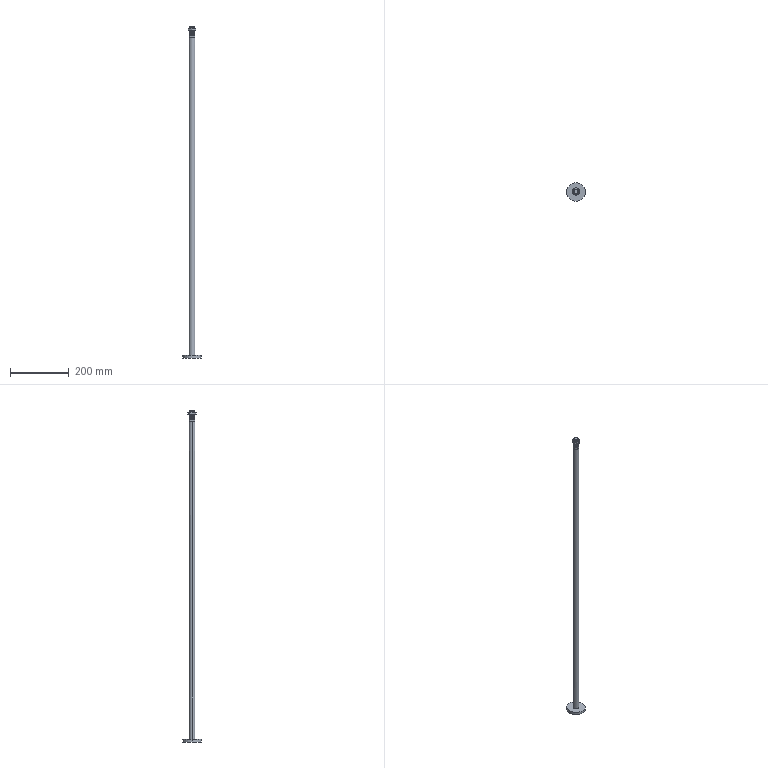Part | SolidWorks | features ICE 5, Revolution 3, RevCut 2, Chamfer 1, Helix 1, LPattern 1, MirrorPattern 1, SweepCut 1 | 1 solid | 78 faces | box 63 x 63 x 1126 mm | volume 379367 mm3 | cylinder 37 | plane 23 | cone 14 | spline 4 | commonest cylinder face diameters 16 x31 14 x2 20 x2 63 x2